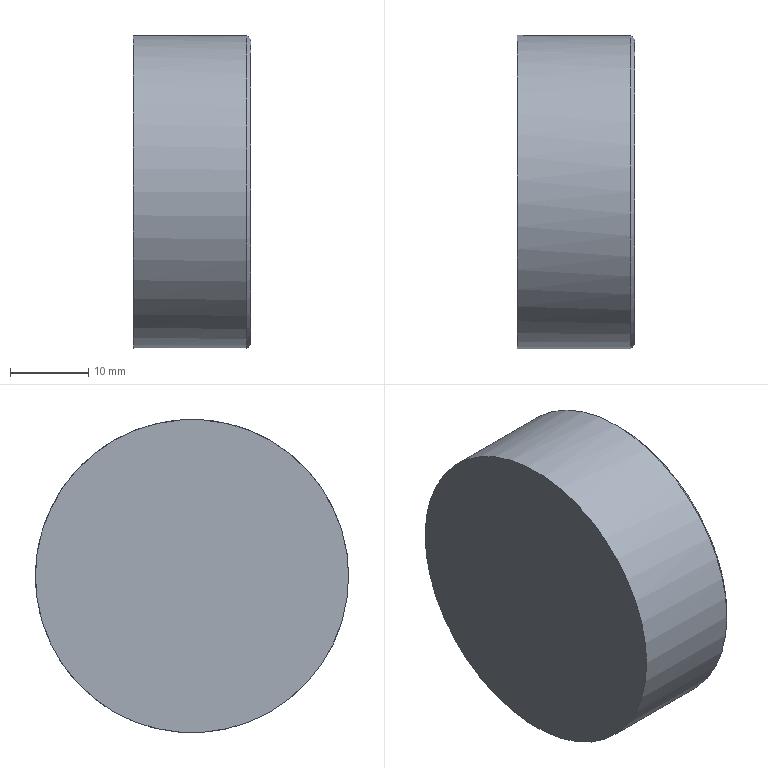Part | STEP file | P0359210003_D | 1 solid | 61 faces | box 15 x 40 x 40 mm | volume 15757 mm3 | cylinder 28 | plane 19 | cone 11 | torus 3 | commonest cylinder face diameters 4.3 x8 5 x8 5.5 x8 2.5 x1 20 x1 20.4 x1